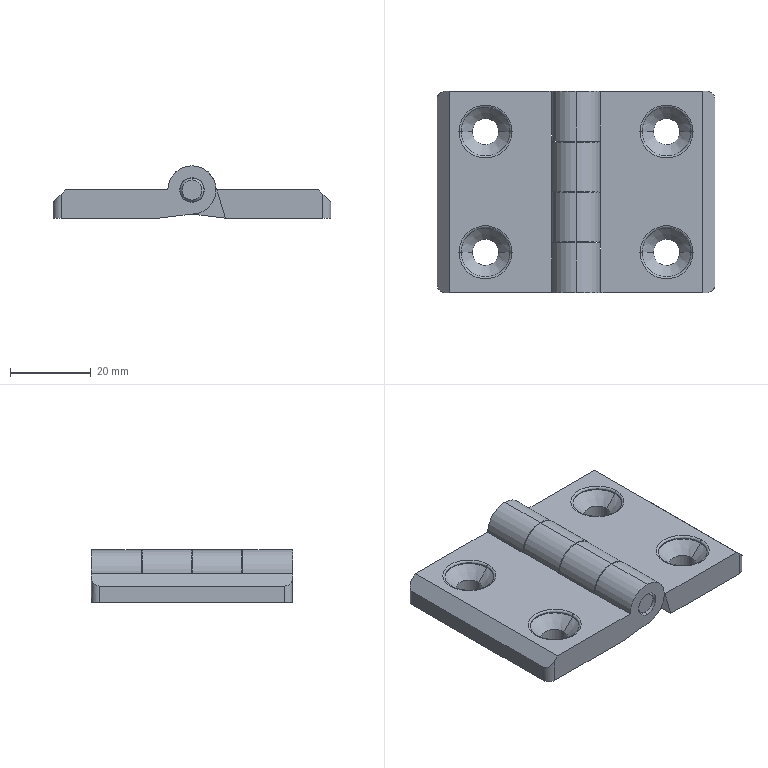Part | SolidWorks | features BaseBody 3 | 3 solids | 93 faces | box 69 x 50 x 13 mm | volume 23385 mm3 | cylinder 36 | plane 29 | torus 16 | cone 12 | commonest cylinder face diameters 6.1 x8 6.5 x8 12 x8 4 x4 10 x4 6 x2